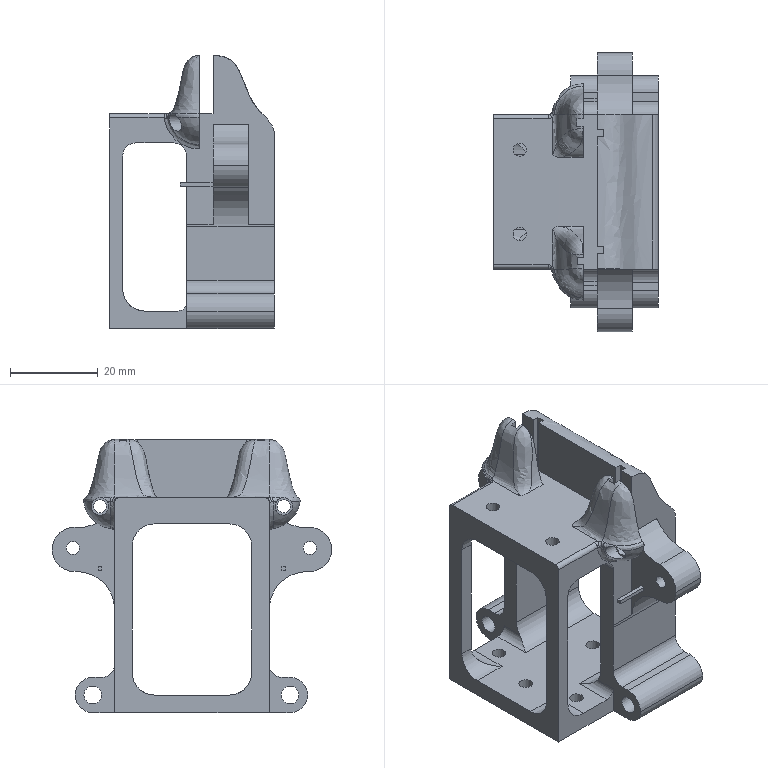Part | STEP file | Lustro3 | 1 solid | 130 faces | box 37.601 x 63.709 x 62.254 mm | volume 29031 mm3 | plane 59 | cylinder 50 | spline 21 | commonest cylinder face diameters 10 x11 2 x6 4 x6 6 x6 3 x4 3.1 x4